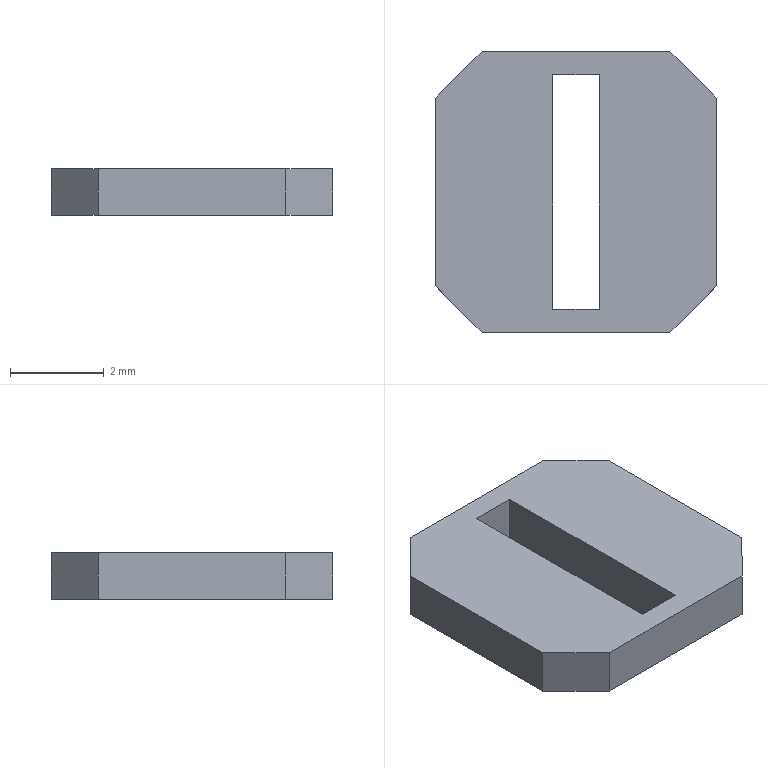Part | STEP file | [OP-85137]-7 | 1 solid | 14 faces | box 6 x 6 x 1 mm | volume 29 mm3 | plane 14
STEP:
#1=CARTESIAN_POINT('',(3.5,0.5,0.));
#2=VERTEX_POINT('',#1);
#3=CARTESIAN_POINT('',(3.5,5.5,0.));
#4=VERTEX_POINT('',#3);
#5=CARTESIAN_POINT('',(3.5,3.,0.));
#6=DIRECTION('',(0.,1.,0.));
#7=VECTOR('',#6,1000.);
#8=LINE('',#5,#7);
#9=EDGE_CURVE('',#2,#4,#8,.T.);
#10=ORIENTED_EDGE('',*,*,#9,.T.);
#11=CARTESIAN_POINT('',(2.5,5.5,0.));
#12=VERTEX_POINT('',#11);
#13=CARTESIAN_POINT('',(3.,5.5,0.));
#14=DIRECTION('',(-1.,0.,0.));
#15=VECTOR('',#14,1000.);
#16=LINE('',#13,#15);
#17=EDGE_CURVE('',#4,#12,#16,.T.);
#18=ORIENTED_EDGE('',*,*,#17,.T.);
#19=CARTESIAN_POINT('',(2.5,0.5,0.));
#20=VERTEX_POINT('',#19);
#21=CARTESIAN_POINT('',(2.5,3.,0.));
#22=DIRECTION('',(0.,-1.,0.));
#23=VECTOR('',#22,1000.);
#24=LINE('',#21,#23);
#25=EDGE_CURVE('',#12,#20,#24,.T.);
#26=ORIENTED_EDGE('',*,*,#25,.T.);
#27=CARTESIAN_POINT('',(3.,0.5,0.));
#28=DIRECTION('',(1.,0.,0.));
#29=VECTOR('',#28,1000.);
#30=LINE('',#27,#29);
#31=EDGE_CURVE('',#20,#2,#30,.T.);
#32=ORIENTED_EDGE('',*,*,#31,.T.);
#33=EDGE_LOOP('',(#10,#18,#26,#32));
#34=FACE_BOUND('',#33,.T.);
#35=CARTESIAN_POINT('',(1.,0.,0.));
#36=VERTEX_POINT('',#35);
#37=CARTESIAN_POINT('',(5.,0.,0.));
#38=VERTEX_POINT('',#37);
#39=CARTESIAN_POINT('',(3.,0.,0.));
#40=DIRECTION('',(1.,0.,0.));
#41=VECTOR('',#40,1000.);
#42=LINE('',#39,#41);
#43=EDGE_CURVE('',#36,#38,#42,.T.);
#44=ORIENTED_EDGE('',*,*,#43,.F.);
#45=CARTESIAN_POINT('',(0.,1.,0.));
#46=VERTEX_POINT('',#45);
#47=CARTESIAN_POINT('',(0.5,0.5,0.));
#48=DIRECTION('',(-0.7071,0.7071,0.));
#49=VECTOR('',#48,1000.);
#50=LINE('',#47,#49);
#51=EDGE_CURVE('',#36,#46,#50,.T.);
#52=ORIENTED_EDGE('',*,*,#51,.T.);
#53=CARTESIAN_POINT('',(0.,5.,0.));
#54=VERTEX_POINT('',#53);
#55=CARTESIAN_POINT('',(0.,3.,0.));
#56=DIRECTION('',(0.,-1.,0.));
#57=VECTOR('',#56,1000.);
#58=LINE('',#55,#57);
#59=EDGE_CURVE('',#54,#46,#58,.T.);
#60=ORIENTED_EDGE('',*,*,#59,.F.);
#61=CARTESIAN_POINT('',(1.,6.,0.));
#62=VERTEX_POINT('',#61);
#63=CARTESIAN_POINT('',(0.5,5.5,0.));
#64=DIRECTION('',(0.7071,0.7071,0.));
#65=VECTOR('',#64,1000.);
#66=LINE('',#63,#65);
#67=EDGE_CURVE('',#54,#62,#66,.T.);
#68=ORIENTED_EDGE('',*,*,#67,.T.);
#69=CARTESIAN_POINT('',(5.,6.,0.));
#70=VERTEX_POINT('',#69);
#71=CARTESIAN_POINT('',(3.,6.,0.));
#72=DIRECTION('',(-1.,0.,0.));
#73=VECTOR('',#72,1000.);
#74=LINE('',#71,#73);
#75=EDGE_CURVE('',#70,#62,#74,.T.);
#76=ORIENTED_EDGE('',*,*,#75,.F.);
#77=CARTESIAN_POINT('',(6.,5.,0.));
#78=VERTEX_POINT('',#77);
#79=CARTESIAN_POINT('',(5.5,5.5,0.));
#80=DIRECTION('',(0.7071,-0.7071,0.));
#81=VECTOR('',#80,1000.);
#82=LINE('',#79,#81);
#83=EDGE_CURVE('',#70,#78,#82,.T.);
#84=ORIENTED_EDGE('',*,*,#83,.T.);
#85=CARTESIAN_POINT('',(6.,1.,0.));
#86=VERTEX_POINT('',#85);
#87=CARTESIAN_POINT('',(6.,3.,0.));
#88=DIRECTION('',(0.,1.,0.));
#89=VECTOR('',#88,1000.);
#90=LINE('',#87,#89);
#91=EDGE_CURVE('',#86,#78,#90,.T.);
#92=ORIENTED_EDGE('',*,*,#91,.F.);
#93=CARTESIAN_POINT('',(5.5,0.5,0.));
#94=DIRECTION('',(-0.7071,-0.7071,0.));
#95=VECTOR('',#94,1000.);
#96=LINE('',#93,#95);
#97=EDGE_CURVE('',#86,#38,#96,.T.);
#98=ORIENTED_EDGE('',*,*,#97,.T.);
#99=EDGE_LOOP('',(#44,#52,#60,#68,#76,#84,#92,#98));
#100=FACE_OUTER_BOUND('',#99,.T.);
#101=CARTESIAN_POINT('',(3.,3.,0.));
#102=DIRECTION('',(0.,0.,-1.));
#103=DIRECTION('',(1.,0.,0.));
#104=AXIS2_PLACEMENT_3D('',#101,#102,#103);
#105=PLANE('',#104);
#106=ADVANCED_FACE('',(#34,#100),#105,.T.);
#107=ORIENTED_EDGE('',*,*,#75,.T.);
#108=CARTESIAN_POINT('',(1.,6.,1.));
#109=VERTEX_POINT('',#108);
#110=CARTESIAN_POINT('',(1.,6.,1.));
#111=DIRECTION('',(0.,0.,1.));
#112=VECTOR('',#111,1000.);
#113=LINE('',#110,#112);
#114=EDGE_CURVE('',#62,#109,#113,.T.);
#115=ORIENTED_EDGE('',*,*,#114,.T.);
#116=CARTESIAN_POINT('',(5.,6.,1.));
#117=VERTEX_POINT('',#116);
#118=CARTESIAN_POINT('',(3.,6.,1.));
#119=DIRECTION('',(1.,0.,0.));
#120=VECTOR('',#119,1000.);
#121=LINE('',#118,#120);
#122=EDGE_CURVE('',#109,#117,#121,.T.);
#123=ORIENTED_EDGE('',*,*,#122,.T.);
#124=CARTESIAN_POINT('',(5.,6.,1.));
#125=DIRECTION('',(0.,0.,-1.));
#126=VECTOR('',#125,1000.);
#127=LINE('',#124,#126);
#128=EDGE_CURVE('',#117,#70,#127,.T.);
#129=ORIENTED_EDGE('',*,*,#128,.T.);
#130=EDGE_LOOP('',(#107,#115,#123,#129));
#131=FACE_OUTER_BOUND('',#130,.T.);
#132=CARTESIAN_POINT('',(3.,6.,1.));
#133=DIRECTION('',(0.,1.,0.));
#134=DIRECTION('',(0.,0.,1.));
#135=AXIS2_PLACEMENT_3D('',#132,#133,#134);
#136=PLANE('',#135);
#137=ADVANCED_FACE('',(#131),#136,.T.);
#138=ORIENTED_EDGE('',*,*,#59,.T.);
#139=CARTESIAN_POINT('',(0.,1.,1.));
#140=VERTEX_POINT('',#139);
#141=CARTESIAN_POINT('',(0.,1.,1.));
#142=DIRECTION('',(0.,0.,1.));
#143=VECTOR('',#142,1000.);
#144=LINE('',#141,#143);
#145=EDGE_CURVE('',#46,#140,#144,.T.);
#146=ORIENTED_EDGE('',*,*,#145,.T.);
#147=CARTESIAN_POINT('',(0.,5.,1.));
#148=VERTEX_POINT('',#147);
#149=CARTESIAN_POINT('',(0.,3.,1.));
#150=DIRECTION('',(0.,1.,0.));
#151=VECTOR('',#150,1000.);
#152=LINE('',#149,#151);
#153=EDGE_CURVE('',#140,#148,#152,.T.);
#154=ORIENTED_EDGE('',*,*,#153,.T.);
#155=CARTESIAN_POINT('',(0.,5.,1.));
#156=DIRECTION('',(0.,0.,-1.));
#157=VECTOR('',#156,1000.);
#158=LINE('',#155,#157);
#159=EDGE_CURVE('',#148,#54,#158,.T.);
#160=ORIENTED_EDGE('',*,*,#159,.T.);
#161=EDGE_LOOP('',(#138,#146,#154,#160));
#162=FACE_OUTER_BOUND('',#161,.T.);
#163=CARTESIAN_POINT('',(0.,3.,1.));
#164=DIRECTION('',(-1.,0.,0.));
#165=DIRECTION('',(0.,0.,-1.));
#166=AXIS2_PLACEMENT_3D('',#163,#164,#165);
#167=PLANE('',#166);
#168=ADVANCED_FACE('',(#162),#167,.T.);
#169=CARTESIAN_POINT('',(5.,0.,1.));
#170=VERTEX_POINT('',#169);
#171=CARTESIAN_POINT('',(1.,0.,1.));
#172=VERTEX_POINT('',#171);
#173=CARTESIAN_POINT('',(3.,0.,1.));
#174=DIRECTION('',(-1.,0.,0.));
#175=VECTOR('',#174,1000.);
#176=LINE('',#173,#175);
#177=EDGE_CURVE('',#170,#172,#176,.T.);
#178=ORIENTED_EDGE('',*,*,#177,.T.);
#179=CARTESIAN_POINT('',(1.,0.,1.));
#180=DIRECTION('',(0.,0.,-1.));
#181=VECTOR('',#180,1000.);
#182=LINE('',#179,#181);
#183=EDGE_CURVE('',#172,#36,#182,.T.);
#184=ORIENTED_EDGE('',*,*,#183,.T.);
#185=ORIENTED_EDGE('',*,*,#43,.T.);
#186=CARTESIAN_POINT('',(5.,0.,1.));
#187=DIRECTION('',(0.,0.,1.));
#188=VECTOR('',#187,1000.);
#189=LINE('',#186,#188);
#190=EDGE_CURVE('',#38,#170,#189,.T.);
#191=ORIENTED_EDGE('',*,*,#190,.T.);
#192=EDGE_LOOP('',(#178,#184,#185,#191));
#193=FACE_OUTER_BOUND('',#192,.T.);
#194=CARTESIAN_POINT('',(3.,0.,1.));
#195=DIRECTION('',(0.,-1.,0.));
#196=DIRECTION('',(0.,0.,-1.));
#197=AXIS2_PLACEMENT_3D('',#194,#195,#196);
#198=PLANE('',#197);
#199=ADVANCED_FACE('',(#193),#198,.T.);
#200=CARTESIAN_POINT('',(3.5,5.5,1.));
#201=VERTEX_POINT('',#200);
#202=CARTESIAN_POINT('',(3.5,0.5,1.));
#203=VERTEX_POINT('',#202);
#204=CARTESIAN_POINT('',(3.5,3.,1.));
#205=DIRECTION('',(0.,-1.,0.));
#206=VECTOR('',#205,1000.);
#207=LINE('',#204,#206);
#208=EDGE_CURVE('',#201,#203,#207,.T.);
#209=ORIENTED_EDGE('',*,*,#208,.T.);
#210=CARTESIAN_POINT('',(2.5,0.5,1.));
#211=VERTEX_POINT('',#210);
#212=CARTESIAN_POINT('',(3.,0.5,1.));
#213=DIRECTION('',(-1.,0.,0.));
#214=VECTOR('',#213,1000.);
#215=LINE('',#212,#214);
#216=EDGE_CURVE('',#203,#211,#215,.T.);
#217=ORIENTED_EDGE('',*,*,#216,.T.);
#218=CARTESIAN_POINT('',(2.5,5.5,1.));
#219=VERTEX_POINT('',#218);
#220=CARTESIAN_POINT('',(2.5,3.,1.));
#221=DIRECTION('',(0.,1.,0.));
#222=VECTOR('',#221,1000.);
#223=LINE('',#220,#222);
#224=EDGE_CURVE('',#211,#219,#223,.T.);
#225=ORIENTED_EDGE('',*,*,#224,.T.);
#226=CARTESIAN_POINT('',(3.,5.5,1.));
#227=DIRECTION('',(1.,0.,0.));
#228=VECTOR('',#227,1000.);
#229=LINE('',#226,#228);
#230=EDGE_CURVE('',#219,#201,#229,.T.);
#231=ORIENTED_EDGE('',*,*,#230,.T.);
#232=EDGE_LOOP('',(#209,#217,#225,#231));
#233=FACE_BOUND('',#232,.T.);
#234=ORIENTED_EDGE('',*,*,#153,.F.);
#235=CARTESIAN_POINT('',(0.5,0.5,1.));
#236=DIRECTION('',(0.7071,-0.7071,0.));
#237=VECTOR('',#236,1000.);
#238=LINE('',#235,#237);
#239=EDGE_CURVE('',#140,#172,#238,.T.);
#240=ORIENTED_EDGE('',*,*,#239,.T.);
#241=ORIENTED_EDGE('',*,*,#177,.F.);
#242=CARTESIAN_POINT('',(6.,1.,1.));
#243=VERTEX_POINT('',#242);
#244=CARTESIAN_POINT('',(5.5,0.5,1.));
#245=DIRECTION('',(0.7071,0.7071,0.));
#246=VECTOR('',#245,1000.);
#247=LINE('',#244,#246);
#248=EDGE_CURVE('',#170,#243,#247,.T.);
#249=ORIENTED_EDGE('',*,*,#248,.T.);
#250=CARTESIAN_POINT('',(6.,5.,1.));
#251=VERTEX_POINT('',#250);
#252=CARTESIAN_POINT('',(6.,3.,1.));
#253=DIRECTION('',(0.,-1.,0.));
#254=VECTOR('',#253,1000.);
#255=LINE('',#252,#254);
#256=EDGE_CURVE('',#251,#243,#255,.T.);
#257=ORIENTED_EDGE('',*,*,#256,.F.);
#258=CARTESIAN_POINT('',(5.5,5.5,1.));
#259=DIRECTION('',(-0.7071,0.7071,0.));
#260=VECTOR('',#259,1000.);
#261=LINE('',#258,#260);
#262=EDGE_CURVE('',#251,#117,#261,.T.);
#263=ORIENTED_EDGE('',*,*,#262,.T.);
#264=ORIENTED_EDGE('',*,*,#122,.F.);
#265=CARTESIAN_POINT('',(0.5,5.5,1.));
#266=DIRECTION('',(-0.7071,-0.7071,0.));
#267=VECTOR('',#266,1000.);
#268=LINE('',#265,#267);
#269=EDGE_CURVE('',#109,#148,#268,.T.);
#270=ORIENTED_EDGE('',*,*,#269,.T.);
#271=EDGE_LOOP('',(#234,#240,#241,#249,#257,#263,#264,#270));
#272=FACE_OUTER_BOUND('',#271,.T.);
#273=CARTESIAN_POINT('',(3.,3.,1.));
#274=DIRECTION('',(0.,0.,1.));
#275=DIRECTION('',(-1.,0.,0.));
#276=AXIS2_PLACEMENT_3D('',#273,#274,#275);
#277=PLANE('',#276);
#278=ADVANCED_FACE('',(#233,#272),#277,.T.);
#279=ORIENTED_EDGE('',*,*,#91,.T.);
#280=CARTESIAN_POINT('',(6.,5.,1.));
#281=DIRECTION('',(0.,0.,1.));
#282=VECTOR('',#281,1000.);
#283=LINE('',#280,#282);
#284=EDGE_CURVE('',#78,#251,#283,.T.);
#285=ORIENTED_EDGE('',*,*,#284,.T.);
#286=ORIENTED_EDGE('',*,*,#256,.T.);
#287=CARTESIAN_POINT('',(6.,1.,1.));
#288=DIRECTION('',(0.,0.,-1.));
#289=VECTOR('',#288,1000.);
#290=LINE('',#287,#289);
#291=EDGE_CURVE('',#243,#86,#290,.T.);
#292=ORIENTED_EDGE('',*,*,#291,.T.);
#293=EDGE_LOOP('',(#279,#285,#286,#292));
#294=FACE_OUTER_BOUND('',#293,.T.);
#295=CARTESIAN_POINT('',(6.,3.,1.));
#296=DIRECTION('',(1.,0.,0.));
#297=DIRECTION('',(0.,0.,1.));
#298=AXIS2_PLACEMENT_3D('',#295,#296,#297);
#299=PLANE('',#298);
#300=ADVANCED_FACE('',(#294),#299,.T.);
#301=CARTESIAN_POINT('',(3.5,5.5,0.));
#302=DIRECTION('',(0.,0.,1.));
#303=VECTOR('',#302,1000.);
#304=LINE('',#301,#303);
#305=EDGE_CURVE('',#4,#201,#304,.T.);
#306=ORIENTED_EDGE('',*,*,#305,.F.);
#307=ORIENTED_EDGE('',*,*,#9,.F.);
#308=CARTESIAN_POINT('',(3.5,0.5,0.));
#309=DIRECTION('',(0.,0.,1.));
#310=VECTOR('',#309,1000.);
#311=LINE('',#308,#310);
#312=EDGE_CURVE('',#2,#203,#311,.T.);
#313=ORIENTED_EDGE('',*,*,#312,.T.);
#314=ORIENTED_EDGE('',*,*,#208,.F.);
#315=EDGE_LOOP('',(#306,#307,#313,#314));
#316=FACE_OUTER_BOUND('',#315,.T.);
#317=CARTESIAN_POINT('',(3.5,3.,0.));
#318=DIRECTION('',(1.,0.,0.));
#319=DIRECTION('',(0.,0.,-1.));
#320=AXIS2_PLACEMENT_3D('',#317,#318,#319);
#321=PLANE('',#320);
#322=ADVANCED_FACE('',(#316),#321,.F.);
#323=ORIENTED_EDGE('',*,*,#312,.F.);
#324=ORIENTED_EDGE('',*,*,#31,.F.);
#325=CARTESIAN_POINT('',(2.5,0.5,0.));
#326=DIRECTION('',(0.,0.,1.));
#327=VECTOR('',#326,1000.);
#328=LINE('',#325,#327);
#329=EDGE_CURVE('',#20,#211,#328,.T.);
#330=ORIENTED_EDGE('',*,*,#329,.T.);
#331=ORIENTED_EDGE('',*,*,#216,.F.);
#332=EDGE_LOOP('',(#323,#324,#330,#331));
#333=FACE_OUTER_BOUND('',#332,.T.);
#334=CARTESIAN_POINT('',(3.,0.5,0.));
#335=DIRECTION('',(0.,-1.,0.));
#336=DIRECTION('',(0.,0.,1.));
#337=AXIS2_PLACEMENT_3D('',#334,#335,#336);
#338=PLANE('',#337);
#339=ADVANCED_FACE('',(#333),#338,.F.);
#340=ORIENTED_EDGE('',*,*,#329,.F.);
#341=ORIENTED_EDGE('',*,*,#25,.F.);
#342=CARTESIAN_POINT('',(2.5,5.5,0.));
#343=DIRECTION('',(0.,0.,1.));
#344=VECTOR('',#343,1000.);
#345=LINE('',#342,#344);
#346=EDGE_CURVE('',#12,#219,#345,.T.);
#347=ORIENTED_EDGE('',*,*,#346,.T.);
#348=ORIENTED_EDGE('',*,*,#224,.F.);
#349=EDGE_LOOP('',(#340,#341,#347,#348));
#350=FACE_OUTER_BOUND('',#349,.T.);
#351=CARTESIAN_POINT('',(2.5,3.,0.));
#352=DIRECTION('',(-1.,0.,0.));
#353=DIRECTION('',(0.,0.,1.));
#354=AXIS2_PLACEMENT_3D('',#351,#352,#353);
#355=PLANE('',#354);
#356=ADVANCED_FACE('',(#350),#355,.F.);
#357=ORIENTED_EDGE('',*,*,#17,.F.);
#358=ORIENTED_EDGE('',*,*,#305,.T.);
#359=ORIENTED_EDGE('',*,*,#230,.F.);
#360=ORIENTED_EDGE('',*,*,#346,.F.);
#361=EDGE_LOOP('',(#357,#358,#359,#360));
#362=FACE_OUTER_BOUND('',#361,.T.);
#363=CARTESIAN_POINT('',(3.,5.5,0.));
#364=DIRECTION('',(0.,1.,0.));
#365=DIRECTION('',(0.,0.,-1.));
#366=AXIS2_PLACEMENT_3D('',#363,#364,#365);
#367=PLANE('',#366);
#368=ADVANCED_FACE('',(#362),#367,.F.);
#369=ORIENTED_EDGE('',*,*,#248,.F.);
#370=ORIENTED_EDGE('',*,*,#190,.F.);
#371=ORIENTED_EDGE('',*,*,#97,.F.);
#372=ORIENTED_EDGE('',*,*,#291,.F.);
#373=EDGE_LOOP('',(#369,#370,#371,#372));
#374=FACE_OUTER_BOUND('',#373,.T.);
#375=CARTESIAN_POINT('',(6.,1.,1.));
#376=DIRECTION('',(-0.7071,0.7071,0.));
#377=DIRECTION('',(0.,0.,-1.));
#378=AXIS2_PLACEMENT_3D('',#375,#376,#377);
#379=PLANE('',#378);
#380=ADVANCED_FACE('',(#374),#379,.F.);
#381=ORIENTED_EDGE('',*,*,#262,.F.);
#382=ORIENTED_EDGE('',*,*,#284,.F.);
#383=ORIENTED_EDGE('',*,*,#83,.F.);
#384=ORIENTED_EDGE('',*,*,#128,.F.);
#385=EDGE_LOOP('',(#381,#382,#383,#384));
#386=FACE_OUTER_BOUND('',#385,.T.);
#387=CARTESIAN_POINT('',(5.,6.,1.));
#388=DIRECTION('',(-0.7071,-0.7071,0.));
#389=DIRECTION('',(0.,0.,-1.));
#390=AXIS2_PLACEMENT_3D('',#387,#388,#389);
#391=PLANE('',#390);
#392=ADVANCED_FACE('',(#386),#391,.F.);
#393=ORIENTED_EDGE('',*,*,#269,.F.);
#394=ORIENTED_EDGE('',*,*,#114,.F.);
#395=ORIENTED_EDGE('',*,*,#67,.F.);
#396=ORIENTED_EDGE('',*,*,#159,.F.);
#397=EDGE_LOOP('',(#393,#394,#395,#396));
#398=FACE_OUTER_BOUND('',#397,.T.);
#399=CARTESIAN_POINT('',(0.,5.,1.));
#400=DIRECTION('',(0.7071,-0.7071,0.));
#401=DIRECTION('',(0.,0.,-1.));
#402=AXIS2_PLACEMENT_3D('',#399,#400,#401);
#403=PLANE('',#402);
#404=ADVANCED_FACE('',(#398),#403,.F.);
#405=ORIENTED_EDGE('',*,*,#239,.F.);
#406=ORIENTED_EDGE('',*,*,#145,.F.);
#407=ORIENTED_EDGE('',*,*,#51,.F.);
#408=ORIENTED_EDGE('',*,*,#183,.F.);
#409=EDGE_LOOP('',(#405,#406,#407,#408));
#410=FACE_OUTER_BOUND('',#409,.T.);
#411=CARTESIAN_POINT('',(1.,0.,1.));
#412=DIRECTION('',(0.7071,0.7071,0.));
#413=DIRECTION('',(0.,0.,-1.));
#414=AXIS2_PLACEMENT_3D('',#411,#412,#413);
#415=PLANE('',#414);
#416=ADVANCED_FACE('',(#410),#415,.F.);
#417=CLOSED_SHELL('',(#106,#137,#168,#199,#278,#300,#322,#339,#356,#368,#380,#392,#404,#416));
#418=MANIFOLD_SOLID_BREP('',#417);
#419=CARTESIAN_POINT('',(0.,0.,0.));
#420=DIRECTION('',(0.,0.,1.));
#421=DIRECTION('',(1.,0.,0.));
#422=AXIS2_PLACEMENT_3D('',#419,#420,#421);
#423=(LENGTH_UNIT()NAMED_UNIT(*)SI_UNIT(.MILLI.,.METRE.));
#424=UNCERTAINTY_MEASURE_WITH_UNIT(LENGTH_MEASURE(0.00001),#423,'','');
#425=(NAMED_UNIT(*)PLANE_ANGLE_UNIT()SI_UNIT($,.RADIAN.));
#426=(NAMED_UNIT(*)SI_UNIT($,.STERADIAN.)SOLID_ANGLE_UNIT());
#427=(GEOMETRIC_REPRESENTATION_CONTEXT(3)GLOBAL_UNCERTAINTY_ASSIGNED_CONTEXT((#424))GLOBAL_UNIT_ASSIGNED_CONTEXT((#423,#425,#426))REPRESENTATION_CONTEXT('',''));
#428=ADVANCED_BREP_SHAPE_REPRESENTATION('',(#418,#422),#427);